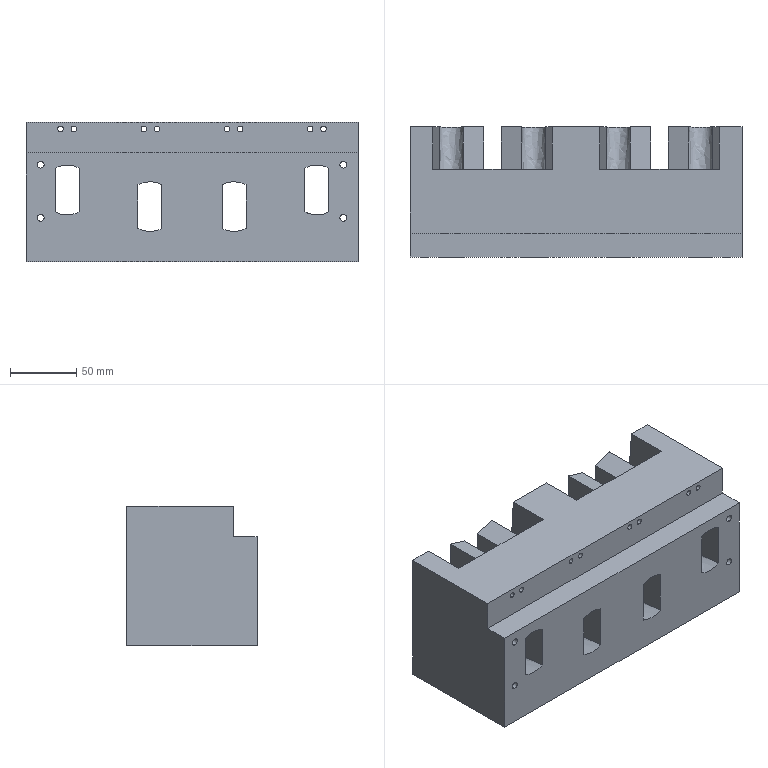Part | 1 solid | 144 faces | box 250 x 98 x 105 mm | volume 1873514 mm3 | cylinder 64 | plane 40 | cone 32 | spline 8 | commonest cylinder face diameters 4.2 x48 5.2 x8 9 x8